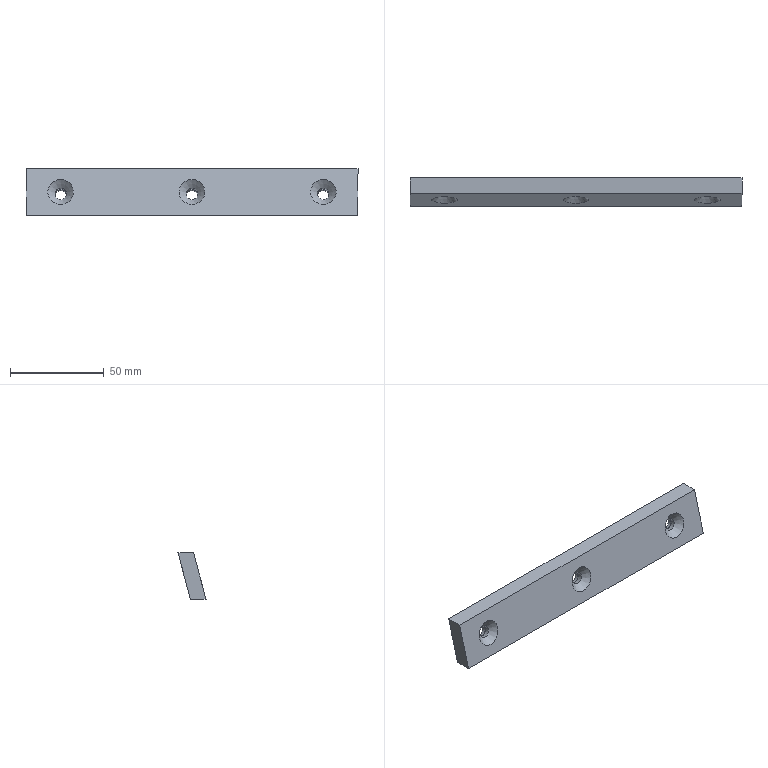Part | STEP file | solid 145 | 1 solid | 18 faces | box 177 x 14.981 x 25 mm | volume 35338 mm3 | plane 9 | cylinder 6 | cone 3 | commonest cylinder face diameters 6 x3 6.5 x3